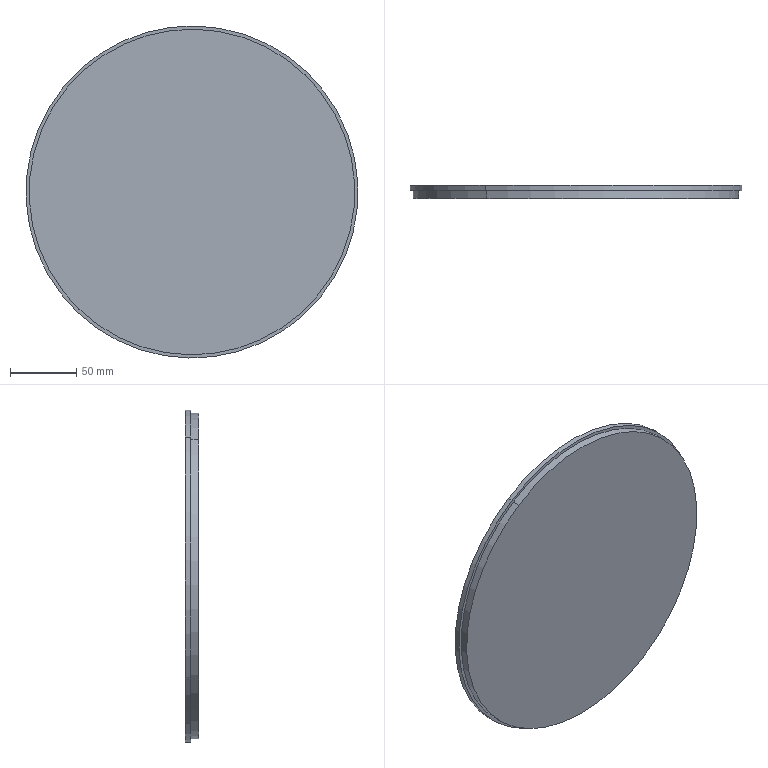Part | STEP file | 1 solid | 7 faces | box 249.9 x 9.8 x 249.9 mm | volume 469473 mm3 | cylinder 4 | plane 3 | commonest cylinder face diameters 245 x2 249.9 x2
STEP:
#1=CARTESIAN_POINT('',(0.,0.,0.));
#2=DIRECTION('',(0.,0.,1.));
#3=DIRECTION('',(1.,0.,0.));
#4=AXIS2_PLACEMENT_3D('',#1,#2,#3);
#5=CARTESIAN_POINT('',(1017.04,-58.309,59.209));
#6=VERTEX_POINT('',#5);
#7=CARTESIAN_POINT('',(883.039,-58.309,264.315));
#8=VERTEX_POINT('',#7);
#9=CARTESIAN_POINT('',(950.039,-58.309,161.762));
#10=DIRECTION('',(0.,-1.,0.));
#11=DIRECTION('',(-0.5469,0.,0.8372));
#12=AXIS2_PLACEMENT_3D('',#9,#10,#11);
#13=CIRCLE('',#12,122.5);
#14=CARTESIAN_POINT('',(950.039,-58.309,161.762));
#15=DIRECTION('',(0.,-1.,0.));
#16=DIRECTION('',(-0.8372,0.,-0.5469));
#17=AXIS2_PLACEMENT_3D('',#14,#15,#16);
#18=PLANE('',#17);
#19=CARTESIAN_POINT('',(0.,0.));
#20=DIRECTION('',(0.,-1.));
#21=AXIS2_PLACEMENT_2D('',#19,#20);
#22=CIRCLE('',#21,122.5);
#23=(GEOMETRIC_REPRESENTATION_CONTEXT(2)PARAMETRIC_REPRESENTATION_CONTEXT()REPRESENTATION_CONTEXT('',''));
#24=DEFINITIONAL_REPRESENTATION('',(#22),#23);
#25=PCURVE('',#18,#24);
#26=CARTESIAN_POINT('',(950.039,-58.309,161.762));
#27=DIRECTION('',(0.,1.,0.));
#28=DIRECTION('',(0.5469,0.,-0.8372));
#29=AXIS2_PLACEMENT_3D('',#26,#27,#28);
#30=CYLINDRICAL_SURFACE('',#29,122.5);
#31=CARTESIAN_POINT('',(9.425,0.));
#32=DIRECTION('',(-1.,0.));
#33=VECTOR('',#32,1.);
#34=LINE('',#31,#33);
#35=(GEOMETRIC_REPRESENTATION_CONTEXT(2)PARAMETRIC_REPRESENTATION_CONTEXT()REPRESENTATION_CONTEXT('',''));
#36=DEFINITIONAL_REPRESENTATION('',(#34),#35);
#37=PCURVE('',#30,#36);
#38=SURFACE_CURVE('',#13,(#25,#37),.PCURVE_S1.);
#39=EDGE_CURVE('',#6,#8,#38,.T.);
#40=ORIENTED_EDGE('',*,*,#39,.T.);
#41=CARTESIAN_POINT('',(950.039,-58.309,161.762));
#42=DIRECTION('',(0.,-1.,0.));
#43=DIRECTION('',(-0.5469,0.,0.8372));
#44=AXIS2_PLACEMENT_3D('',#41,#42,#43);
#45=CIRCLE('',#44,122.5);
#46=CARTESIAN_POINT('',(0.,0.));
#47=DIRECTION('',(0.,-1.));
#48=AXIS2_PLACEMENT_2D('',#46,#47);
#49=CIRCLE('',#48,122.5);
#50=(GEOMETRIC_REPRESENTATION_CONTEXT(2)PARAMETRIC_REPRESENTATION_CONTEXT()REPRESENTATION_CONTEXT('',''));
#51=DEFINITIONAL_REPRESENTATION('',(#49),#50);
#52=PCURVE('',#18,#51);
#53=CARTESIAN_POINT('',(950.039,-58.309,161.762));
#54=DIRECTION('',(0.,1.,0.));
#55=DIRECTION('',(0.5469,0.,-0.8372));
#56=AXIS2_PLACEMENT_3D('',#53,#54,#55);
#57=CYLINDRICAL_SURFACE('',#56,122.5);
#58=CARTESIAN_POINT('',(3.142,0.));
#59=DIRECTION('',(-1.,0.));
#60=VECTOR('',#59,1.);
#61=LINE('',#58,#60);
#62=(GEOMETRIC_REPRESENTATION_CONTEXT(2)PARAMETRIC_REPRESENTATION_CONTEXT()REPRESENTATION_CONTEXT('',''));
#63=DEFINITIONAL_REPRESENTATION('',(#61),#62);
#64=PCURVE('',#57,#63);
#65=SURFACE_CURVE('',#45,(#52,#64),.PCURVE_S1.);
#66=EDGE_CURVE('',#8,#6,#65,.T.);
#67=ORIENTED_EDGE('',*,*,#66,.T.);
#68=EDGE_LOOP('',(#40,#67));
#69=FACE_BOUND('',#68,.T.);
#70=ADVANCED_FACE('',(#69),#18,.T.);
#71=CARTESIAN_POINT('',(883.039,-52.429,264.315));
#72=VERTEX_POINT('',#71);
#73=CARTESIAN_POINT('',(883.039,-58.309,264.315));
#74=DIRECTION('',(0.,1.,0.));
#75=VECTOR('',#74,1.);
#76=LINE('',#73,#75);
#77=CARTESIAN_POINT('',(3.142,0.));
#78=DIRECTION('',(0.,1.));
#79=VECTOR('',#78,1.);
#80=LINE('',#77,#79);
#81=(GEOMETRIC_REPRESENTATION_CONTEXT(2)PARAMETRIC_REPRESENTATION_CONTEXT()REPRESENTATION_CONTEXT('',''));
#82=DEFINITIONAL_REPRESENTATION('',(#80),#81);
#83=PCURVE('',#30,#82);
#84=CARTESIAN_POINT('',(3.142,0.));
#85=DIRECTION('',(0.,1.));
#86=VECTOR('',#85,1.);
#87=LINE('',#84,#86);
#88=(GEOMETRIC_REPRESENTATION_CONTEXT(2)PARAMETRIC_REPRESENTATION_CONTEXT()REPRESENTATION_CONTEXT('',''));
#89=DEFINITIONAL_REPRESENTATION('',(#87),#88);
#90=PCURVE('',#57,#89);
#91=SURFACE_CURVE('',#76,(#83,#90),.PCURVE_S1.);
#92=EDGE_CURVE('',#8,#72,#91,.T.);
#93=ORIENTED_EDGE('',*,*,#92,.F.);
#94=ORIENTED_EDGE('',*,*,#39,.F.);
#95=CARTESIAN_POINT('',(1017.04,-52.429,59.209));
#96=VERTEX_POINT('',#95);
#97=CARTESIAN_POINT('',(1017.04,-58.309,59.209));
#98=DIRECTION('',(0.,1.,0.));
#99=VECTOR('',#98,1.);
#100=LINE('',#97,#99);
#101=CARTESIAN_POINT('',(6.283,0.));
#102=DIRECTION('',(0.,1.));
#103=VECTOR('',#102,1.);
#104=LINE('',#101,#103);
#105=(GEOMETRIC_REPRESENTATION_CONTEXT(2)PARAMETRIC_REPRESENTATION_CONTEXT()REPRESENTATION_CONTEXT('',''));
#106=DEFINITIONAL_REPRESENTATION('',(#104),#105);
#107=PCURVE('',#30,#106);
#108=CARTESIAN_POINT('',(0.,0.));
#109=DIRECTION('',(0.,1.));
#110=VECTOR('',#109,1.);
#111=LINE('',#108,#110);
#112=(GEOMETRIC_REPRESENTATION_CONTEXT(2)PARAMETRIC_REPRESENTATION_CONTEXT()REPRESENTATION_CONTEXT('',''));
#113=DEFINITIONAL_REPRESENTATION('',(#111),#112);
#114=PCURVE('',#57,#113);
#115=SURFACE_CURVE('',#100,(#107,#114),.PCURVE_S1.);
#116=EDGE_CURVE('',#6,#96,#115,.T.);
#117=ORIENTED_EDGE('',*,*,#116,.T.);
#118=CARTESIAN_POINT('',(950.039,-52.429,161.762));
#119=DIRECTION('',(0.,-1.,0.));
#120=DIRECTION('',(-0.5469,0.,0.8372));
#121=AXIS2_PLACEMENT_3D('',#118,#119,#120);
#122=CIRCLE('',#121,122.5);
#123=CARTESIAN_POINT('',(9.425,5.88));
#124=DIRECTION('',(-1.,0.));
#125=VECTOR('',#124,1.);
#126=LINE('',#123,#125);
#127=(GEOMETRIC_REPRESENTATION_CONTEXT(2)PARAMETRIC_REPRESENTATION_CONTEXT()REPRESENTATION_CONTEXT('',''));
#128=DEFINITIONAL_REPRESENTATION('',(#126),#127);
#129=PCURVE('',#30,#128);
#130=CARTESIAN_POINT('',(950.039,-52.429,161.762));
#131=DIRECTION('',(0.,-1.,0.));
#132=DIRECTION('',(-0.8372,0.,-0.5469));
#133=AXIS2_PLACEMENT_3D('',#130,#131,#132);
#134=PLANE('',#133);
#135=CARTESIAN_POINT('',(0.,0.));
#136=DIRECTION('',(0.,-1.));
#137=AXIS2_PLACEMENT_2D('',#135,#136);
#138=CIRCLE('',#137,122.5);
#139=(GEOMETRIC_REPRESENTATION_CONTEXT(2)PARAMETRIC_REPRESENTATION_CONTEXT()REPRESENTATION_CONTEXT('',''));
#140=DEFINITIONAL_REPRESENTATION('',(#138),#139);
#141=PCURVE('',#134,#140);
#142=SURFACE_CURVE('',#122,(#129,#141),.PCURVE_S1.);
#143=EDGE_CURVE('',#96,#72,#142,.T.);
#144=ORIENTED_EDGE('',*,*,#143,.T.);
#145=EDGE_LOOP('',(#93,#94,#117,#144));
#146=FACE_BOUND('',#145,.T.);
#147=ADVANCED_FACE('',(#146),#30,.T.);
#148=CARTESIAN_POINT('',(1018.38,-48.509,57.158));
#149=VERTEX_POINT('',#148);
#150=CARTESIAN_POINT('',(881.699,-48.509,266.366));
#151=VERTEX_POINT('',#150);
#152=CARTESIAN_POINT('',(950.039,-48.509,161.762));
#153=DIRECTION('',(0.,-1.,0.));
#154=DIRECTION('',(-0.5469,0.,0.8372));
#155=AXIS2_PLACEMENT_3D('',#152,#153,#154);
#156=CIRCLE('',#155,124.95);
#157=CARTESIAN_POINT('',(950.039,-48.509,161.762));
#158=DIRECTION('',(0.,-1.,0.));
#159=DIRECTION('',(-0.8372,0.,-0.5469));
#160=AXIS2_PLACEMENT_3D('',#157,#158,#159);
#161=PLANE('',#160);
#162=CARTESIAN_POINT('',(0.,0.));
#163=DIRECTION('',(0.,-1.));
#164=AXIS2_PLACEMENT_2D('',#162,#163);
#165=CIRCLE('',#164,124.95);
#166=(GEOMETRIC_REPRESENTATION_CONTEXT(2)PARAMETRIC_REPRESENTATION_CONTEXT()REPRESENTATION_CONTEXT('',''));
#167=DEFINITIONAL_REPRESENTATION('',(#165),#166);
#168=PCURVE('',#161,#167);
#169=CARTESIAN_POINT('',(950.039,-52.429,161.762));
#170=DIRECTION('',(0.,1.,0.));
#171=DIRECTION('',(0.5469,0.,-0.8372));
#172=AXIS2_PLACEMENT_3D('',#169,#170,#171);
#173=CYLINDRICAL_SURFACE('',#172,124.95);
#174=CARTESIAN_POINT('',(9.425,3.92));
#175=DIRECTION('',(-1.,0.));
#176=VECTOR('',#175,1.);
#177=LINE('',#174,#176);
#178=(GEOMETRIC_REPRESENTATION_CONTEXT(2)PARAMETRIC_REPRESENTATION_CONTEXT()REPRESENTATION_CONTEXT('',''));
#179=DEFINITIONAL_REPRESENTATION('',(#177),#178);
#180=PCURVE('',#173,#179);
#181=SURFACE_CURVE('',#156,(#168,#180),.PCURVE_S1.);
#182=EDGE_CURVE('',#149,#151,#181,.T.);
#183=ORIENTED_EDGE('',*,*,#182,.F.);
#184=CARTESIAN_POINT('',(950.039,-48.509,161.762));
#185=DIRECTION('',(0.,-1.,0.));
#186=DIRECTION('',(-0.5469,0.,0.8372));
#187=AXIS2_PLACEMENT_3D('',#184,#185,#186);
#188=CIRCLE('',#187,124.95);
#189=CARTESIAN_POINT('',(0.,0.));
#190=DIRECTION('',(0.,-1.));
#191=AXIS2_PLACEMENT_2D('',#189,#190);
#192=CIRCLE('',#191,124.95);
#193=(GEOMETRIC_REPRESENTATION_CONTEXT(2)PARAMETRIC_REPRESENTATION_CONTEXT()REPRESENTATION_CONTEXT('',''));
#194=DEFINITIONAL_REPRESENTATION('',(#192),#193);
#195=PCURVE('',#161,#194);
#196=CARTESIAN_POINT('',(950.039,-52.429,161.762));
#197=DIRECTION('',(0.,1.,0.));
#198=DIRECTION('',(0.5469,0.,-0.8372));
#199=AXIS2_PLACEMENT_3D('',#196,#197,#198);
#200=CYLINDRICAL_SURFACE('',#199,124.95);
#201=CARTESIAN_POINT('',(3.142,3.92));
#202=DIRECTION('',(-1.,0.));
#203=VECTOR('',#202,1.);
#204=LINE('',#201,#203);
#205=(GEOMETRIC_REPRESENTATION_CONTEXT(2)PARAMETRIC_REPRESENTATION_CONTEXT()REPRESENTATION_CONTEXT('',''));
#206=DEFINITIONAL_REPRESENTATION('',(#204),#205);
#207=PCURVE('',#200,#206);
#208=SURFACE_CURVE('',#188,(#195,#207),.PCURVE_S1.);
#209=EDGE_CURVE('',#151,#149,#208,.T.);
#210=ORIENTED_EDGE('',*,*,#209,.F.);
#211=EDGE_LOOP('',(#183,#210));
#212=FACE_BOUND('',#211,.T.);
#213=ADVANCED_FACE('',(#212),#161,.F.);
#214=ORIENTED_EDGE('',*,*,#143,.F.);
#215=CARTESIAN_POINT('',(950.039,-52.429,161.762));
#216=DIRECTION('',(0.,-1.,0.));
#217=DIRECTION('',(-0.5469,0.,0.8372));
#218=AXIS2_PLACEMENT_3D('',#215,#216,#217);
#219=CIRCLE('',#218,122.5);
#220=CARTESIAN_POINT('',(0.,0.));
#221=DIRECTION('',(0.,-1.));
#222=AXIS2_PLACEMENT_2D('',#220,#221);
#223=CIRCLE('',#222,122.5);
#224=(GEOMETRIC_REPRESENTATION_CONTEXT(2)PARAMETRIC_REPRESENTATION_CONTEXT()REPRESENTATION_CONTEXT('',''));
#225=DEFINITIONAL_REPRESENTATION('',(#223),#224);
#226=PCURVE('',#134,#225);
#227=CARTESIAN_POINT('',(3.142,5.88));
#228=DIRECTION('',(-1.,0.));
#229=VECTOR('',#228,1.);
#230=LINE('',#227,#229);
#231=(GEOMETRIC_REPRESENTATION_CONTEXT(2)PARAMETRIC_REPRESENTATION_CONTEXT()REPRESENTATION_CONTEXT('',''));
#232=DEFINITIONAL_REPRESENTATION('',(#230),#231);
#233=PCURVE('',#57,#232);
#234=SURFACE_CURVE('',#219,(#226,#233),.PCURVE_S1.);
#235=EDGE_CURVE('',#72,#96,#234,.T.);
#236=ORIENTED_EDGE('',*,*,#235,.F.);
#237=EDGE_LOOP('',(#214,#236));
#238=FACE_BOUND('',#237,.T.);
#239=CARTESIAN_POINT('',(1018.38,-52.429,57.158));
#240=VERTEX_POINT('',#239);
#241=CARTESIAN_POINT('',(881.699,-52.429,266.366));
#242=VERTEX_POINT('',#241);
#243=CARTESIAN_POINT('',(950.039,-52.429,161.762));
#244=DIRECTION('',(0.,-1.,0.));
#245=DIRECTION('',(-0.5469,0.,0.8372));
#246=AXIS2_PLACEMENT_3D('',#243,#244,#245);
#247=CIRCLE('',#246,124.95);
#248=CARTESIAN_POINT('',(0.,0.));
#249=DIRECTION('',(0.,-1.));
#250=AXIS2_PLACEMENT_2D('',#248,#249);
#251=CIRCLE('',#250,124.95);
#252=(GEOMETRIC_REPRESENTATION_CONTEXT(2)PARAMETRIC_REPRESENTATION_CONTEXT()REPRESENTATION_CONTEXT('',''));
#253=DEFINITIONAL_REPRESENTATION('',(#251),#252);
#254=PCURVE('',#134,#253);
#255=CARTESIAN_POINT('',(9.425,0.));
#256=DIRECTION('',(-1.,0.));
#257=VECTOR('',#256,1.);
#258=LINE('',#255,#257);
#259=(GEOMETRIC_REPRESENTATION_CONTEXT(2)PARAMETRIC_REPRESENTATION_CONTEXT()REPRESENTATION_CONTEXT('',''));
#260=DEFINITIONAL_REPRESENTATION('',(#258),#259);
#261=PCURVE('',#173,#260);
#262=SURFACE_CURVE('',#247,(#254,#261),.PCURVE_S1.);
#263=EDGE_CURVE('',#240,#242,#262,.T.);
#264=ORIENTED_EDGE('',*,*,#263,.T.);
#265=CARTESIAN_POINT('',(950.039,-52.429,161.762));
#266=DIRECTION('',(0.,-1.,0.));
#267=DIRECTION('',(-0.5469,0.,0.8372));
#268=AXIS2_PLACEMENT_3D('',#265,#266,#267);
#269=CIRCLE('',#268,124.95);
#270=CARTESIAN_POINT('',(0.,0.));
#271=DIRECTION('',(0.,-1.));
#272=AXIS2_PLACEMENT_2D('',#270,#271);
#273=CIRCLE('',#272,124.95);
#274=(GEOMETRIC_REPRESENTATION_CONTEXT(2)PARAMETRIC_REPRESENTATION_CONTEXT()REPRESENTATION_CONTEXT('',''));
#275=DEFINITIONAL_REPRESENTATION('',(#273),#274);
#276=PCURVE('',#134,#275);
#277=CARTESIAN_POINT('',(3.142,0.));
#278=DIRECTION('',(-1.,0.));
#279=VECTOR('',#278,1.);
#280=LINE('',#277,#279);
#281=(GEOMETRIC_REPRESENTATION_CONTEXT(2)PARAMETRIC_REPRESENTATION_CONTEXT()REPRESENTATION_CONTEXT('',''));
#282=DEFINITIONAL_REPRESENTATION('',(#280),#281);
#283=PCURVE('',#200,#282);
#284=SURFACE_CURVE('',#269,(#276,#283),.PCURVE_S1.);
#285=EDGE_CURVE('',#242,#240,#284,.T.);
#286=ORIENTED_EDGE('',*,*,#285,.T.);
#287=EDGE_LOOP('',(#264,#286));
#288=FACE_BOUND('',#287,.T.);
#289=ADVANCED_FACE('',(#238,#288),#134,.T.);
#290=CARTESIAN_POINT('',(881.699,-52.429,266.366));
#291=DIRECTION('',(0.,1.,0.));
#292=VECTOR('',#291,1.);
#293=LINE('',#290,#292);
#294=CARTESIAN_POINT('',(3.142,0.));
#295=DIRECTION('',(0.,1.));
#296=VECTOR('',#295,1.);
#297=LINE('',#294,#296);
#298=(GEOMETRIC_REPRESENTATION_CONTEXT(2)PARAMETRIC_REPRESENTATION_CONTEXT()REPRESENTATION_CONTEXT('',''));
#299=DEFINITIONAL_REPRESENTATION('',(#297),#298);
#300=PCURVE('',#173,#299);
#301=CARTESIAN_POINT('',(3.142,0.));
#302=DIRECTION('',(0.,1.));
#303=VECTOR('',#302,1.);
#304=LINE('',#301,#303);
#305=(GEOMETRIC_REPRESENTATION_CONTEXT(2)PARAMETRIC_REPRESENTATION_CONTEXT()REPRESENTATION_CONTEXT('',''));
#306=DEFINITIONAL_REPRESENTATION('',(#304),#305);
#307=PCURVE('',#200,#306);
#308=SURFACE_CURVE('',#293,(#300,#307),.PCURVE_S1.);
#309=EDGE_CURVE('',#242,#151,#308,.T.);
#310=ORIENTED_EDGE('',*,*,#309,.F.);
#311=ORIENTED_EDGE('',*,*,#263,.F.);
#312=CARTESIAN_POINT('',(1018.38,-52.429,57.158));
#313=DIRECTION('',(0.,1.,0.));
#314=VECTOR('',#313,1.);
#315=LINE('',#312,#314);
#316=CARTESIAN_POINT('',(6.283,0.));
#317=DIRECTION('',(0.,1.));
#318=VECTOR('',#317,1.);
#319=LINE('',#316,#318);
#320=(GEOMETRIC_REPRESENTATION_CONTEXT(2)PARAMETRIC_REPRESENTATION_CONTEXT()REPRESENTATION_CONTEXT('',''));
#321=DEFINITIONAL_REPRESENTATION('',(#319),#320);
#322=PCURVE('',#173,#321);
#323=CARTESIAN_POINT('',(0.,0.));
#324=DIRECTION('',(0.,1.));
#325=VECTOR('',#324,1.);
#326=LINE('',#323,#325);
#327=(GEOMETRIC_REPRESENTATION_CONTEXT(2)PARAMETRIC_REPRESENTATION_CONTEXT()REPRESENTATION_CONTEXT('',''));
#328=DEFINITIONAL_REPRESENTATION('',(#326),#327);
#329=PCURVE('',#200,#328);
#330=SURFACE_CURVE('',#315,(#322,#329),.PCURVE_S1.);
#331=EDGE_CURVE('',#240,#149,#330,.T.);
#332=ORIENTED_EDGE('',*,*,#331,.T.);
#333=ORIENTED_EDGE('',*,*,#182,.T.);
#334=EDGE_LOOP('',(#310,#311,#332,#333));
#335=FACE_BOUND('',#334,.T.);
#336=ADVANCED_FACE('',(#335),#173,.T.);
#337=ORIENTED_EDGE('',*,*,#285,.F.);
#338=ORIENTED_EDGE('',*,*,#309,.T.);
#339=ORIENTED_EDGE('',*,*,#209,.T.);
#340=ORIENTED_EDGE('',*,*,#331,.F.);
#341=EDGE_LOOP('',(#337,#338,#339,#340));
#342=FACE_BOUND('',#341,.T.);
#343=ADVANCED_FACE('',(#342),#200,.T.);
#344=ORIENTED_EDGE('',*,*,#66,.F.);
#345=ORIENTED_EDGE('',*,*,#92,.T.);
#346=ORIENTED_EDGE('',*,*,#235,.T.);
#347=ORIENTED_EDGE('',*,*,#116,.F.);
#348=EDGE_LOOP('',(#344,#345,#346,#347));
#349=FACE_BOUND('',#348,.T.);
#350=ADVANCED_FACE('',(#349),#57,.T.);
#351=CLOSED_SHELL('',(#70,#147,#213,#289,#336,#343,#350));
#352=MANIFOLD_SOLID_BREP('',#351);
#353=(LENGTH_UNIT()NAMED_UNIT(*)SI_UNIT(.MILLI.,.METRE.));
#354=UNCERTAINTY_MEASURE_WITH_UNIT(LENGTH_MEASURE(0.0000001),#353,'','');
#355=(NAMED_UNIT(*)PLANE_ANGLE_UNIT()SI_UNIT($,.RADIAN.));
#356=(NAMED_UNIT(*)SI_UNIT($,.STERADIAN.)SOLID_ANGLE_UNIT());
#357=(GEOMETRIC_REPRESENTATION_CONTEXT(3)GLOBAL_UNCERTAINTY_ASSIGNED_CONTEXT((#354))GLOBAL_UNIT_ASSIGNED_CONTEXT((#353,#355,#356))REPRESENTATION_CONTEXT('',''));
#358=ADVANCED_BREP_SHAPE_REPRESENTATION('',(#4,#352),#357);